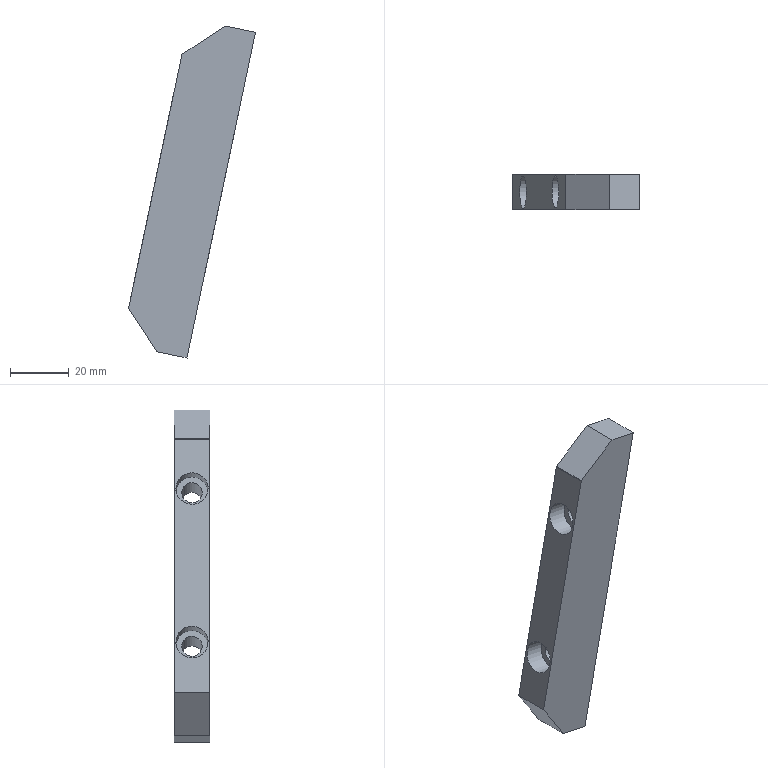Part | STEP file | BERCO_003 | 1 solid | 15 faces | box 43.278 x 12 x 113.233 mm | volume 26889 mm3 | plane 11 | cylinder 4 | commonest cylinder face diameters 7 x2 11 x2
STEP:
#1=CARTESIAN_POINT('',(0.,0.,0.));
#2=DIRECTION('',(0.,0.,1.));
#3=DIRECTION('',(1.,0.,0.));
#4=AXIS2_PLACEMENT_3D('',#1,#2,#3);
#5=CARTESIAN_POINT('',(1194.353,-560.013,65.597));
#6=VERTEX_POINT('',#5);
#7=CARTESIAN_POINT('',(1195.346,-562.65,70.321));
#8=DIRECTION('',(0.9786,0.,-0.2056));
#9=DIRECTION('',(0.2056,0.,0.9786));
#10=AXIS2_PLACEMENT_3D('',#7,#8,#9);
#11=CIRCLE('',#10,5.5);
#12=CARTESIAN_POINT('',(1196.066,-562.65,73.746));
#13=DIRECTION('',(0.9786,0.,-0.2056));
#14=DIRECTION('',(-0.2056,0.,-0.9786));
#15=AXIS2_PLACEMENT_3D('',#12,#13,#14);
#16=PLANE('',#15);
#17=CARTESIAN_POINT('',(3.5,0.));
#18=DIRECTION('',(-1.,0.));
#19=AXIS2_PLACEMENT_2D('',#17,#18);
#20=CIRCLE('',#19,5.5);
#21=(GEOMETRIC_REPRESENTATION_CONTEXT(2)PARAMETRIC_REPRESENTATION_CONTEXT()REPRESENTATION_CONTEXT('',''));
#22=DEFINITIONAL_REPRESENTATION('',(#20),#21);
#23=PCURVE('',#16,#22);
#24=CARTESIAN_POINT('',(1188.593,-562.65,71.74));
#25=DIRECTION('',(0.9786,0.,-0.2056));
#26=DIRECTION('',(0.1805,-0.4794,0.8588));
#27=AXIS2_PLACEMENT_3D('',#24,#25,#26);
#28=CYLINDRICAL_SURFACE('',#27,5.5);
#29=CARTESIAN_POINT('',(-0.5,6.9));
#30=DIRECTION('',(1.,0.));
#31=VECTOR('',#30,1.);
#32=LINE('',#29,#31);
#33=(GEOMETRIC_REPRESENTATION_CONTEXT(2)PARAMETRIC_REPRESENTATION_CONTEXT()REPRESENTATION_CONTEXT('',''));
#34=DEFINITIONAL_REPRESENTATION('',(#32),#33);
#35=PCURVE('',#28,#34);
#36=SURFACE_CURVE('',#11,(#23,#35),.PCURVE_S1.);
#37=EDGE_CURVE('',#6,#6,#36,.T.);
#38=ORIENTED_EDGE('',*,*,#37,.F.);
#39=EDGE_LOOP('',(#38));
#40=FACE_BOUND('',#39,.T.);
#41=CARTESIAN_POINT('',(1195.978,-564.328,73.327));
#42=VERTEX_POINT('',#41);
#43=CARTESIAN_POINT('',(1195.346,-562.65,70.321));
#44=DIRECTION('',(0.9786,0.,-0.2056));
#45=DIRECTION('',(0.2056,0.,0.9786));
#46=AXIS2_PLACEMENT_3D('',#43,#44,#45);
#47=CIRCLE('',#46,3.5);
#48=CARTESIAN_POINT('',(3.5,0.));
#49=DIRECTION('',(-1.,0.));
#50=AXIS2_PLACEMENT_2D('',#48,#49);
#51=CIRCLE('',#50,3.5);
#52=(GEOMETRIC_REPRESENTATION_CONTEXT(2)PARAMETRIC_REPRESENTATION_CONTEXT()REPRESENTATION_CONTEXT('',''));
#53=DEFINITIONAL_REPRESENTATION('',(#51),#52);
#54=PCURVE('',#16,#53);
#55=CARTESIAN_POINT('',(1188.593,-562.65,71.74));
#56=DIRECTION('',(0.9786,0.,-0.2056));
#57=DIRECTION('',(0.1805,-0.4794,0.8588));
#58=AXIS2_PLACEMENT_3D('',#55,#56,#57);
#59=CYLINDRICAL_SURFACE('',#58,3.5);
#60=CARTESIAN_POINT('',(-0.5,6.9));
#61=DIRECTION('',(1.,0.));
#62=VECTOR('',#61,1.);
#63=LINE('',#60,#62);
#64=(GEOMETRIC_REPRESENTATION_CONTEXT(2)PARAMETRIC_REPRESENTATION_CONTEXT()REPRESENTATION_CONTEXT('',''));
#65=DEFINITIONAL_REPRESENTATION('',(#63),#64);
#66=PCURVE('',#59,#65);
#67=SURFACE_CURVE('',#47,(#54,#66),.PCURVE_S1.);
#68=EDGE_CURVE('',#42,#42,#67,.T.);
#69=ORIENTED_EDGE('',*,*,#68,.T.);
#70=EDGE_LOOP('',(#69));
#71=FACE_BOUND('',#70,.T.);
#72=ADVANCED_FACE('',(#40,#71),#16,.F.);
#73=CARTESIAN_POINT('',(1211.636,-564.328,70.036));
#74=VERTEX_POINT('',#73);
#75=CARTESIAN_POINT('',(1211.004,-562.65,67.031));
#76=DIRECTION('',(0.9786,0.,-0.2056));
#77=DIRECTION('',(0.2056,0.,0.9786));
#78=AXIS2_PLACEMENT_3D('',#75,#76,#77);
#79=CIRCLE('',#78,3.5);
#80=CARTESIAN_POINT('',(-0.5,22.9));
#81=DIRECTION('',(1.,0.));
#82=VECTOR('',#81,1.);
#83=LINE('',#80,#82);
#84=(GEOMETRIC_REPRESENTATION_CONTEXT(2)PARAMETRIC_REPRESENTATION_CONTEXT()REPRESENTATION_CONTEXT('',''));
#85=DEFINITIONAL_REPRESENTATION('',(#83),#84);
#86=PCURVE('',#59,#85);
#87=CARTESIAN_POINT('',(1228.175,-556.65,148.746));
#88=DIRECTION('',(-0.9786,0.,0.2056));
#89=DIRECTION('',(0.2056,0.,0.9786));
#90=AXIS2_PLACEMENT_3D('',#87,#88,#89);
#91=PLANE('',#90);
#92=CARTESIAN_POINT('',(-80.,-6.));
#93=CARTESIAN_POINT('',(-80.,-12.062));
#94=CARTESIAN_POINT('',(-85.25,-9.031));
#95=CARTESIAN_POINT('',(-90.5,-6.));
#96=CARTESIAN_POINT('',(-85.25,-2.969));
#97=CARTESIAN_POINT('',(-80.,0.06218));
#98=CARTESIAN_POINT('',(-80.,-6.));
#99=(BOUNDED_CURVE()B_SPLINE_CURVE(2,(#92,#93,#94,#95,#96,#97,#98),.UNSPECIFIED.,.T.,.F.)B_SPLINE_CURVE_WITH_KNOTS((1,2,2,2,2,1),(-2.094,0.,2.094,4.189,6.283,8.378),.UNSPECIFIED.)CURVE()GEOMETRIC_REPRESENTATION_ITEM()RATIONAL_B_SPLINE_CURVE((1.,0.5,1.,0.5,1.,0.5,1.))REPRESENTATION_ITEM(''));
#100=(GEOMETRIC_REPRESENTATION_CONTEXT(2)PARAMETRIC_REPRESENTATION_CONTEXT()REPRESENTATION_CONTEXT('',''));
#101=DEFINITIONAL_REPRESENTATION('',(#99),#100);
#102=PCURVE('',#91,#101);
#103=SURFACE_CURVE('',#79,(#86,#102),.PCURVE_S1.);
#104=EDGE_CURVE('',#74,#74,#103,.T.);
#105=ORIENTED_EDGE('',*,*,#104,.F.);
#106=CARTESIAN_POINT('',(1195.978,-564.328,73.327));
#107=CARTESIAN_POINT('',(1211.636,-564.328,70.036));
#108=B_SPLINE_CURVE_WITH_KNOTS('',1,(#106,#107),.UNSPECIFIED.,.F.,.F.,(2,2),(6.9,22.9),.PIECEWISE_BEZIER_KNOTS.);
#109=CARTESIAN_POINT('',(0.,0.));
#110=DIRECTION('',(0.,1.));
#111=VECTOR('',#110,1.);
#112=LINE('',#109,#111);
#113=(GEOMETRIC_REPRESENTATION_CONTEXT(2)PARAMETRIC_REPRESENTATION_CONTEXT()REPRESENTATION_CONTEXT('',''));
#114=DEFINITIONAL_REPRESENTATION('',(#112),#113);
#115=PCURVE('',#59,#114);
#116=CARTESIAN_POINT('',(6.283,0.));
#117=DIRECTION('',(0.,1.));
#118=VECTOR('',#117,1.);
#119=LINE('',#116,#118);
#120=(GEOMETRIC_REPRESENTATION_CONTEXT(2)PARAMETRIC_REPRESENTATION_CONTEXT()REPRESENTATION_CONTEXT('',''));
#121=DEFINITIONAL_REPRESENTATION('',(#119),#120);
#122=PCURVE('',#59,#121);
#123=SEAM_CURVE('',#108,(#115,#122),.PCURVE_S1.);
#124=EDGE_CURVE('',#42,#74,#123,.T.);
#125=ORIENTED_EDGE('',*,*,#124,.F.);
#126=ORIENTED_EDGE('',*,*,#68,.T.);
#127=ORIENTED_EDGE('',*,*,#124,.T.);
#128=EDGE_LOOP('',(#105,#125,#126,#127));
#129=FACE_BOUND('',#128,.F.);
#130=ADVANCED_FACE('',(#129),#59,.F.);
#131=CARTESIAN_POINT('',(1187.503,-560.013,67.037));
#132=VERTEX_POINT('',#131);
#133=CARTESIAN_POINT('',(1188.496,-562.65,71.76));
#134=DIRECTION('',(0.9786,0.,-0.2056));
#135=DIRECTION('',(0.2056,0.,0.9786));
#136=AXIS2_PLACEMENT_3D('',#133,#134,#135);
#137=CIRCLE('',#136,5.5);
#138=CARTESIAN_POINT('',(-0.5,-0.1));
#139=DIRECTION('',(1.,0.));
#140=VECTOR('',#139,1.);
#141=LINE('',#138,#140);
#142=(GEOMETRIC_REPRESENTATION_CONTEXT(2)PARAMETRIC_REPRESENTATION_CONTEXT()REPRESENTATION_CONTEXT('',''));
#143=DEFINITIONAL_REPRESENTATION('',(#141),#142);
#144=PCURVE('',#28,#143);
#145=CARTESIAN_POINT('',(1184.383,-556.65,52.188));
#146=DIRECTION('',(-0.9786,0.,0.2056));
#147=DIRECTION('',(0.2056,0.,0.9786));
#148=AXIS2_PLACEMENT_3D('',#145,#146,#147);
#149=PLANE('',#148);
#150=CARTESIAN_POINT('',(25.5,-6.));
#151=CARTESIAN_POINT('',(25.5,-15.526));
#152=CARTESIAN_POINT('',(17.25,-10.763));
#153=CARTESIAN_POINT('',(9.,-6.));
#154=CARTESIAN_POINT('',(17.25,-1.237));
#155=CARTESIAN_POINT('',(25.5,3.526));
#156=CARTESIAN_POINT('',(25.5,-6.));
#157=(BOUNDED_CURVE()B_SPLINE_CURVE(2,(#150,#151,#152,#153,#154,#155,#156),.UNSPECIFIED.,.T.,.F.)B_SPLINE_CURVE_WITH_KNOTS((1,2,2,2,2,1),(-2.094,0.,2.094,4.189,6.283,8.378),.UNSPECIFIED.)CURVE()GEOMETRIC_REPRESENTATION_ITEM()RATIONAL_B_SPLINE_CURVE((1.,0.5,1.,0.5,1.,0.5,1.))REPRESENTATION_ITEM(''));
#158=(GEOMETRIC_REPRESENTATION_CONTEXT(2)PARAMETRIC_REPRESENTATION_CONTEXT()REPRESENTATION_CONTEXT('',''));
#159=DEFINITIONAL_REPRESENTATION('',(#157),#158);
#160=PCURVE('',#149,#159);
#161=SURFACE_CURVE('',#137,(#144,#160),.PCURVE_S1.);
#162=EDGE_CURVE('',#132,#132,#161,.T.);
#163=ORIENTED_EDGE('',*,*,#162,.T.);
#164=CARTESIAN_POINT('',(1187.503,-560.013,67.037));
#165=CARTESIAN_POINT('',(1194.353,-560.013,65.597));
#166=B_SPLINE_CURVE_WITH_KNOTS('',1,(#164,#165),.UNSPECIFIED.,.F.,.F.,(2,2),(-0.1,6.9),.PIECEWISE_BEZIER_KNOTS.);
#167=CARTESIAN_POINT('',(9.425,0.));
#168=DIRECTION('',(0.,1.));
#169=VECTOR('',#168,1.);
#170=LINE('',#167,#169);
#171=(GEOMETRIC_REPRESENTATION_CONTEXT(2)PARAMETRIC_REPRESENTATION_CONTEXT()REPRESENTATION_CONTEXT('',''));
#172=DEFINITIONAL_REPRESENTATION('',(#170),#171);
#173=PCURVE('',#28,#172);
#174=CARTESIAN_POINT('',(3.142,0.));
#175=DIRECTION('',(0.,1.));
#176=VECTOR('',#175,1.);
#177=LINE('',#174,#176);
#178=(GEOMETRIC_REPRESENTATION_CONTEXT(2)PARAMETRIC_REPRESENTATION_CONTEXT()REPRESENTATION_CONTEXT('',''));
#179=DEFINITIONAL_REPRESENTATION('',(#177),#178);
#180=PCURVE('',#28,#179);
#181=SEAM_CURVE('',#166,(#173,#180),.PCURVE_S1.);
#182=EDGE_CURVE('',#132,#6,#181,.T.);
#183=ORIENTED_EDGE('',*,*,#182,.T.);
#184=ORIENTED_EDGE('',*,*,#37,.F.);
#185=ORIENTED_EDGE('',*,*,#182,.F.);
#186=EDGE_LOOP('',(#163,#183,#184,#185));
#187=FACE_BOUND('',#186,.F.);
#188=ADVANCED_FACE('',(#187),#28,.F.);
#189=CARTESIAN_POINT('',(1228.175,-568.65,148.746));
#190=VERTEX_POINT('',#189);
#191=CARTESIAN_POINT('',(1204.835,-568.65,37.672));
#192=VERTEX_POINT('',#191);
#193=CARTESIAN_POINT('',(1228.175,-568.65,148.746));
#194=DIRECTION('',(-0.2056,0.,-0.9786));
#195=VECTOR('',#194,1.);
#196=LINE('',#193,#195);
#197=CARTESIAN_POINT('',(0.,-12.));
#198=DIRECTION('',(-1.,0.));
#199=VECTOR('',#198,1.);
#200=LINE('',#197,#199);
#201=(GEOMETRIC_REPRESENTATION_CONTEXT(2)PARAMETRIC_REPRESENTATION_CONTEXT()REPRESENTATION_CONTEXT('',''));
#202=DEFINITIONAL_REPRESENTATION('',(#200),#201);
#203=PCURVE('',#91,#202);
#204=CARTESIAN_POINT('',(0.,-568.65,0.));
#205=DIRECTION('',(0.,1.,0.));
#206=DIRECTION('',(0.,0.,1.));
#207=AXIS2_PLACEMENT_3D('',#204,#205,#206);
#208=PLANE('',#207);
#209=CARTESIAN_POINT('',(148.746,1228.175));
#210=DIRECTION('',(-0.9786,-0.2056));
#211=VECTOR('',#210,1.);
#212=LINE('',#209,#211);
#213=(GEOMETRIC_REPRESENTATION_CONTEXT(2)PARAMETRIC_REPRESENTATION_CONTEXT()REPRESENTATION_CONTEXT('',''));
#214=DEFINITIONAL_REPRESENTATION('',(#212),#213);
#215=PCURVE('',#208,#214);
#216=SURFACE_CURVE('',#196,(#203,#215),.PCURVE_S1.);
#217=EDGE_CURVE('',#190,#192,#216,.T.);
#218=ORIENTED_EDGE('',*,*,#217,.T.);
#219=CARTESIAN_POINT('',(1204.835,-556.65,37.672));
#220=VERTEX_POINT('',#219);
#221=CARTESIAN_POINT('',(1204.835,-556.65,37.672));
#222=DIRECTION('',(0.,-1.,0.));
#223=VECTOR('',#222,1.);
#224=LINE('',#221,#223);
#225=CARTESIAN_POINT('',(-113.5,0.));
#226=DIRECTION('',(0.,-1.));
#227=VECTOR('',#226,1.);
#228=LINE('',#225,#227);
#229=(GEOMETRIC_REPRESENTATION_CONTEXT(2)PARAMETRIC_REPRESENTATION_CONTEXT()REPRESENTATION_CONTEXT('',''));
#230=DEFINITIONAL_REPRESENTATION('',(#228),#229);
#231=PCURVE('',#91,#230);
#232=CARTESIAN_POINT('',(1192.113,-556.65,40.345));
#233=DIRECTION('',(-0.2056,0.,-0.9786));
#234=DIRECTION('',(-0.9786,0.,0.2056));
#235=AXIS2_PLACEMENT_3D('',#232,#233,#234);
#236=PLANE('',#235);
#237=CARTESIAN_POINT('',(-13.,0.));
#238=DIRECTION('',(0.,-1.));
#239=VECTOR('',#238,1.);
#240=LINE('',#237,#239);
#241=(GEOMETRIC_REPRESENTATION_CONTEXT(2)PARAMETRIC_REPRESENTATION_CONTEXT()REPRESENTATION_CONTEXT('',''));
#242=DEFINITIONAL_REPRESENTATION('',(#240),#241);
#243=PCURVE('',#236,#242);
#244=SURFACE_CURVE('',#224,(#231,#243),.PCURVE_S1.);
#245=EDGE_CURVE('',#220,#192,#244,.T.);
#246=ORIENTED_EDGE('',*,*,#245,.F.);
#247=CARTESIAN_POINT('',(1228.175,-556.65,148.746));
#248=VERTEX_POINT('',#247);
#249=CARTESIAN_POINT('',(1228.175,-556.65,148.746));
#250=DIRECTION('',(-0.2056,0.,-0.9786));
#251=VECTOR('',#250,1.);
#252=LINE('',#249,#251);
#253=CARTESIAN_POINT('',(0.,0.));
#254=DIRECTION('',(-1.,0.));
#255=VECTOR('',#254,1.);
#256=LINE('',#253,#255);
#257=(GEOMETRIC_REPRESENTATION_CONTEXT(2)PARAMETRIC_REPRESENTATION_CONTEXT()REPRESENTATION_CONTEXT('',''));
#258=DEFINITIONAL_REPRESENTATION('',(#256),#257);
#259=PCURVE('',#91,#258);
#260=CARTESIAN_POINT('',(0.,-556.65,0.));
#261=DIRECTION('',(0.,1.,0.));
#262=DIRECTION('',(0.,0.,1.));
#263=AXIS2_PLACEMENT_3D('',#260,#261,#262);
#264=PLANE('',#263);
#265=CARTESIAN_POINT('',(148.746,1228.175));
#266=DIRECTION('',(-0.9786,-0.2056));
#267=VECTOR('',#266,1.);
#268=LINE('',#265,#267);
#269=(GEOMETRIC_REPRESENTATION_CONTEXT(2)PARAMETRIC_REPRESENTATION_CONTEXT()REPRESENTATION_CONTEXT('',''));
#270=DEFINITIONAL_REPRESENTATION('',(#268),#269);
#271=PCURVE('',#264,#270);
#272=SURFACE_CURVE('',#252,(#259,#271),.PCURVE_S1.);
#273=EDGE_CURVE('',#248,#220,#272,.T.);
#274=ORIENTED_EDGE('',*,*,#273,.F.);
#275=CARTESIAN_POINT('',(1228.175,-556.65,148.746));
#276=DIRECTION('',(0.,-1.,0.));
#277=VECTOR('',#276,1.);
#278=LINE('',#275,#277);
#279=CARTESIAN_POINT('',(0.,0.));
#280=DIRECTION('',(0.,-1.));
#281=VECTOR('',#280,1.);
#282=LINE('',#279,#281);
#283=(GEOMETRIC_REPRESENTATION_CONTEXT(2)PARAMETRIC_REPRESENTATION_CONTEXT()REPRESENTATION_CONTEXT('',''));
#284=DEFINITIONAL_REPRESENTATION('',(#282),#283);
#285=PCURVE('',#91,#284);
#286=CARTESIAN_POINT('',(1205.667,-556.65,153.476));
#287=DIRECTION('',(-0.2056,0.,-0.9786));
#288=DIRECTION('',(-0.9786,0.,0.2056));
#289=AXIS2_PLACEMENT_3D('',#286,#287,#288);
#290=PLANE('',#289);
#291=CARTESIAN_POINT('',(-23.,0.));
#292=DIRECTION('',(0.,-1.));
#293=VECTOR('',#292,1.);
#294=LINE('',#291,#293);
#295=(GEOMETRIC_REPRESENTATION_CONTEXT(2)PARAMETRIC_REPRESENTATION_CONTEXT()REPRESENTATION_CONTEXT('',''));
#296=DEFINITIONAL_REPRESENTATION('',(#294),#295);
#297=PCURVE('',#290,#296);
#298=SURFACE_CURVE('',#278,(#285,#297),.PCURVE_S1.);
#299=EDGE_CURVE('',#248,#190,#298,.T.);
#300=ORIENTED_EDGE('',*,*,#299,.T.);
#301=EDGE_LOOP('',(#218,#246,#274,#300));
#302=FACE_BOUND('',#301,.T.);
#303=CARTESIAN_POINT('',(1222.638,-564.328,122.393));
#304=VERTEX_POINT('',#303);
#305=CARTESIAN_POINT('',(1222.006,-562.65,119.387));
#306=DIRECTION('',(-0.9786,0.,0.2056));
#307=DIRECTION('',(0.2056,0.,0.9786));
#308=AXIS2_PLACEMENT_3D('',#305,#306,#307);
#309=CIRCLE('',#308,3.5);
#310=CARTESIAN_POINT('',(-30.,-6.));
#311=DIRECTION('',(1.,0.));
#312=AXIS2_PLACEMENT_2D('',#310,#311);
#313=CIRCLE('',#312,3.5);
#314=(GEOMETRIC_REPRESENTATION_CONTEXT(2)PARAMETRIC_REPRESENTATION_CONTEXT()REPRESENTATION_CONTEXT('',''));
#315=DEFINITIONAL_REPRESENTATION('',(#313),#314);
#316=PCURVE('',#91,#315);
#317=CARTESIAN_POINT('',(1199.595,-562.65,124.096));
#318=DIRECTION('',(0.9786,0.,-0.2056));
#319=DIRECTION('',(0.1805,-0.4794,0.8588));
#320=AXIS2_PLACEMENT_3D('',#317,#318,#319);
#321=CYLINDRICAL_SURFACE('',#320,3.5);
#322=CARTESIAN_POINT('',(12.066,22.9));
#323=DIRECTION('',(-1.,0.));
#324=VECTOR('',#323,1.);
#325=LINE('',#322,#324);
#326=(GEOMETRIC_REPRESENTATION_CONTEXT(2)PARAMETRIC_REPRESENTATION_CONTEXT()REPRESENTATION_CONTEXT('',''));
#327=DEFINITIONAL_REPRESENTATION('',(#325),#326);
#328=PCURVE('',#321,#327);
#329=SURFACE_CURVE('',#309,(#316,#328),.PCURVE_S1.);
#330=EDGE_CURVE('',#304,#304,#329,.T.);
#331=ORIENTED_EDGE('',*,*,#330,.T.);
#332=EDGE_LOOP('',(#331));
#333=FACE_BOUND('',#332,.T.);
#334=ORIENTED_EDGE('',*,*,#104,.F.);
#335=EDGE_LOOP('',(#334));
#336=FACE_BOUND('',#335,.T.);
#337=ADVANCED_FACE('',(#302,#333,#336),#91,.F.);
#338=CARTESIAN_POINT('',(1207.34,-565.287,127.401));
#339=VERTEX_POINT('',#338);
#340=CARTESIAN_POINT('',(1206.348,-562.65,122.677));
#341=DIRECTION('',(0.9786,0.,-0.2056));
#342=DIRECTION('',(0.2056,0.,0.9786));
#343=AXIS2_PLACEMENT_3D('',#340,#341,#342);
#344=CIRCLE('',#343,5.5);
#345=CARTESIAN_POINT('',(1196.066,-562.65,73.746));
#346=DIRECTION('',(0.9786,0.,-0.2056));
#347=DIRECTION('',(-0.2056,0.,-0.9786));
#348=AXIS2_PLACEMENT_3D('',#345,#346,#347);
#349=PLANE('',#348);
#350=CARTESIAN_POINT('',(-50.,0.));
#351=DIRECTION('',(-1.,0.));
#352=AXIS2_PLACEMENT_2D('',#350,#351);
#353=CIRCLE('',#352,5.5);
#354=(GEOMETRIC_REPRESENTATION_CONTEXT(2)PARAMETRIC_REPRESENTATION_CONTEXT()REPRESENTATION_CONTEXT('',''));
#355=DEFINITIONAL_REPRESENTATION('',(#353),#354);
#356=PCURVE('',#349,#355);
#357=CARTESIAN_POINT('',(1199.595,-562.65,124.096));
#358=DIRECTION('',(0.9786,0.,-0.2056));
#359=DIRECTION('',(0.1805,-0.4794,0.8588));
#360=AXIS2_PLACEMENT_3D('',#357,#358,#359);
#361=CYLINDRICAL_SURFACE('',#360,5.5);
#362=CARTESIAN_POINT('',(-0.5,6.9));
#363=DIRECTION('',(1.,0.));
#364=VECTOR('',#363,1.);
#365=LINE('',#362,#364);
#366=(GEOMETRIC_REPRESENTATION_CONTEXT(2)PARAMETRIC_REPRESENTATION_CONTEXT()REPRESENTATION_CONTEXT('',''));
#367=DEFINITIONAL_REPRESENTATION('',(#365),#366);
#368=PCURVE('',#361,#367);
#369=SURFACE_CURVE('',#344,(#356,#368),.PCURVE_S1.);
#370=EDGE_CURVE('',#339,#339,#369,.T.);
#371=ORIENTED_EDGE('',*,*,#370,.F.);
#372=EDGE_LOOP('',(#371));
#373=FACE_BOUND('',#372,.T.);
#374=CARTESIAN_POINT('',(1206.98,-564.328,125.683));
#375=VERTEX_POINT('',#374);
#376=CARTESIAN_POINT('',(1206.348,-562.65,122.677));
#377=DIRECTION('',(0.9786,0.,-0.2056));
#378=DIRECTION('',(0.2056,0.,0.9786));
#379=AXIS2_PLACEMENT_3D('',#376,#377,#378);
#380=CIRCLE('',#379,3.5);
#381=CARTESIAN_POINT('',(-50.,0.));
#382=DIRECTION('',(-1.,0.));
#383=AXIS2_PLACEMENT_2D('',#381,#382);
#384=CIRCLE('',#383,3.5);
#385=(GEOMETRIC_REPRESENTATION_CONTEXT(2)PARAMETRIC_REPRESENTATION_CONTEXT()REPRESENTATION_CONTEXT('',''));
#386=DEFINITIONAL_REPRESENTATION('',(#384),#385);
#387=PCURVE('',#349,#386);
#388=CARTESIAN_POINT('',(-0.5,6.9));
#389=DIRECTION('',(1.,0.));
#390=VECTOR('',#389,1.);
#391=LINE('',#388,#390);
#392=(GEOMETRIC_REPRESENTATION_CONTEXT(2)PARAMETRIC_REPRESENTATION_CONTEXT()REPRESENTATION_CONTEXT('',''));
#393=DEFINITIONAL_REPRESENTATION('',(#391),#392);
#394=PCURVE('',#321,#393);
#395=SURFACE_CURVE('',#380,(#387,#394),.PCURVE_S1.);
#396=EDGE_CURVE('',#375,#375,#395,.T.);
#397=ORIENTED_EDGE('',*,*,#396,.T.);
#398=EDGE_LOOP('',(#397));
#399=FACE_BOUND('',#398,.T.);
#400=ADVANCED_FACE('',(#373,#399),#349,.F.);
#401=CARTESIAN_POINT('',(1200.49,-565.287,128.84));
#402=VERTEX_POINT('',#401);
#403=CARTESIAN_POINT('',(1199.497,-562.65,124.117));
#404=DIRECTION('',(0.9786,0.,-0.2056));
#405=DIRECTION('',(0.2056,0.,0.9786));
#406=AXIS2_PLACEMENT_3D('',#403,#404,#405);
#407=CIRCLE('',#406,5.5);
#408=CARTESIAN_POINT('',(-0.5,-0.1));
#409=DIRECTION('',(1.,0.));
#410=VECTOR('',#409,1.);
#411=LINE('',#408,#410);
#412=(GEOMETRIC_REPRESENTATION_CONTEXT(2)PARAMETRIC_REPRESENTATION_CONTEXT()REPRESENTATION_CONTEXT('',''));
#413=DEFINITIONAL_REPRESENTATION('',(#411),#412);
#414=PCURVE('',#361,#413);
#415=CARTESIAN_POINT('',(79.,-6.));
#416=CARTESIAN_POINT('',(79.,-15.526));
#417=CARTESIAN_POINT('',(70.75,-10.763));
#418=CARTESIAN_POINT('',(62.5,-6.));
#419=CARTESIAN_POINT('',(70.75,-1.237));
#420=CARTESIAN_POINT('',(79.,3.526));
#421=CARTESIAN_POINT('',(79.,-6.));
#422=(BOUNDED_CURVE()B_SPLINE_CURVE(2,(#415,#416,#417,#418,#419,#420,#421),.UNSPECIFIED.,.T.,.F.)B_SPLINE_CURVE_WITH_KNOTS((1,2,2,2,2,1),(-2.094,0.,2.094,4.189,6.283,8.378),.UNSPECIFIED.)CURVE()GEOMETRIC_REPRESENTATION_ITEM()RATIONAL_B_SPLINE_CURVE((1.,0.5,1.,0.5,1.,0.5,1.))REPRESENTATION_ITEM(''));
#423=(GEOMETRIC_REPRESENTATION_CONTEXT(2)PARAMETRIC_REPRESENTATION_CONTEXT()REPRESENTATION_CONTEXT('',''));
#424=DEFINITIONAL_REPRESENTATION('',(#422),#423);
#425=PCURVE('',#149,#424);
#426=SURFACE_CURVE('',#407,(#414,#425),.PCURVE_S1.);
#427=EDGE_CURVE('',#402,#402,#426,.T.);
#428=ORIENTED_EDGE('',*,*,#427,.T.);
#429=CARTESIAN_POINT('',(1200.49,-565.287,128.84));
#430=CARTESIAN_POINT('',(1207.34,-565.287,127.401));
#431=B_SPLINE_CURVE_WITH_KNOTS('',1,(#429,#430),.UNSPECIFIED.,.F.,.F.,(2,2),(-0.1,6.9),.PIECEWISE_BEZIER_KNOTS.);
#432=CARTESIAN_POINT('',(6.283,0.));
#433=DIRECTION('',(0.,1.));
#434=VECTOR('',#433,1.);
#435=LINE('',#432,#434);
#436=(GEOMETRIC_REPRESENTATION_CONTEXT(2)PARAMETRIC_REPRESENTATION_CONTEXT()REPRESENTATION_CONTEXT('',''));
#437=DEFINITIONAL_REPRESENTATION('',(#435),#436);
#438=PCURVE('',#361,#437);
#439=CARTESIAN_POINT('',(0.,0.));
#440=DIRECTION('',(0.,1.));
#441=VECTOR('',#440,1.);
#442=LINE('',#439,#441);
#443=(GEOMETRIC_REPRESENTATION_CONTEXT(2)PARAMETRIC_REPRESENTATION_CONTEXT()REPRESENTATION_CONTEXT('',''));
#444=DEFINITIONAL_REPRESENTATION('',(#442),#443);
#445=PCURVE('',#361,#444);
#446=SEAM_CURVE('',#431,(#438,#445),.PCURVE_S1.);
#447=EDGE_CURVE('',#402,#339,#446,.T.);
#448=ORIENTED_EDGE('',*,*,#447,.T.);
#449=ORIENTED_EDGE('',*,*,#370,.F.);
#450=ORIENTED_EDGE('',*,*,#447,.F.);
#451=EDGE_LOOP('',(#428,#448,#449,#450));
#452=FACE_BOUND('',#451,.F.);
#453=ADVANCED_FACE('',(#452),#361,.F.);
#454=ORIENTED_EDGE('',*,*,#330,.T.);
#455=CARTESIAN_POINT('',(1206.98,-564.328,125.683));
#456=CARTESIAN_POINT('',(1222.638,-564.328,122.393));
#457=B_SPLINE_CURVE_WITH_KNOTS('',1,(#455,#456),.UNSPECIFIED.,.F.,.F.,(2,2),(6.9,22.9),.PIECEWISE_BEZIER_KNOTS.);
#458=CARTESIAN_POINT('',(0.,0.));
#459=DIRECTION('',(0.,1.));
#460=VECTOR('',#459,1.);
#461=LINE('',#458,#460);
#462=(GEOMETRIC_REPRESENTATION_CONTEXT(2)PARAMETRIC_REPRESENTATION_CONTEXT()REPRESENTATION_CONTEXT('',''));
#463=DEFINITIONAL_REPRESENTATION('',(#461),#462);
#464=PCURVE('',#321,#463);
#465=CARTESIAN_POINT('',(6.283,0.));
#466=DIRECTION('',(0.,1.));
#467=VECTOR('',#466,1.);
#468=LINE('',#465,#467);
#469=(GEOMETRIC_REPRESENTATION_CONTEXT(2)PARAMETRIC_REPRESENTATION_CONTEXT()REPRESENTATION_CONTEXT('',''));
#470=DEFINITIONAL_REPRESENTATION('',(#468),#469);
#471=PCURVE('',#321,#470);
#472=SEAM_CURVE('',#457,(#464,#471),.PCURVE_S1.);
#473=EDGE_CURVE('',#375,#304,#472,.T.);
#474=ORIENTED_EDGE('',*,*,#473,.F.);
#475=ORIENTED_EDGE('',*,*,#396,.T.);
#476=ORIENTED_EDGE('',*,*,#473,.T.);
#477=EDGE_LOOP('',(#454,#474,#475,#476));
#478=FACE_BOUND('',#477,.F.);
#479=ADVANCED_FACE('',(#478),#321,.F.);
#480=CARTESIAN_POINT('',(1217.9,-556.65,150.905));
#481=VERTEX_POINT('',#480);
#482=CARTESIAN_POINT('',(1217.9,-568.65,150.905));
#483=VERTEX_POINT('',#482);
#484=CARTESIAN_POINT('',(1217.9,-556.65,150.905));
#485=DIRECTION('',(0.,-1.,0.));
#486=VECTOR('',#485,1.);
#487=LINE('',#484,#486);
#488=CARTESIAN_POINT('',(-12.5,0.));
#489=DIRECTION('',(0.,-1.));
#490=VECTOR('',#489,1.);
#491=LINE('',#488,#490);
#492=(GEOMETRIC_REPRESENTATION_CONTEXT(2)PARAMETRIC_REPRESENTATION_CONTEXT()REPRESENTATION_CONTEXT('',''));
#493=DEFINITIONAL_REPRESENTATION('',(#491),#492);
#494=PCURVE('',#290,#493);
#495=CARTESIAN_POINT('',(1203.096,-554.25,141.243));
#496=DIRECTION('',(-0.5466,0.,0.8374));
#497=DIRECTION('',(0.8374,0.,0.5466));
#498=AXIS2_PLACEMENT_3D('',#495,#496,#497);
#499=PLANE('',#498);
#500=CARTESIAN_POINT('',(17.678,-2.4));
#501=DIRECTION('',(0.,-1.));
#502=VECTOR('',#501,1.);
#503=LINE('',#500,#502);
#504=(GEOMETRIC_REPRESENTATION_CONTEXT(2)PARAMETRIC_REPRESENTATION_CONTEXT()REPRESENTATION_CONTEXT('',''));
#505=DEFINITIONAL_REPRESENTATION('',(#503),#504);
#506=PCURVE('',#499,#505);
#507=SURFACE_CURVE('',#487,(#494,#506),.PCURVE_S1.);
#508=EDGE_CURVE('',#481,#483,#507,.T.);
#509=ORIENTED_EDGE('',*,*,#508,.T.);
#510=CARTESIAN_POINT('',(1217.9,-568.65,150.905));
#511=DIRECTION('',(0.9786,0.,-0.2056));
#512=VECTOR('',#511,1.);
#513=LINE('',#510,#512);
#514=CARTESIAN_POINT('',(-12.5,-12.));
#515=DIRECTION('',(-1.,0.));
#516=VECTOR('',#515,1.);
#517=LINE('',#514,#516);
#518=(GEOMETRIC_REPRESENTATION_CONTEXT(2)PARAMETRIC_REPRESENTATION_CONTEXT()REPRESENTATION_CONTEXT('',''));
#519=DEFINITIONAL_REPRESENTATION('',(#517),#518);
#520=PCURVE('',#290,#519);
#521=CARTESIAN_POINT('',(150.905,1217.9));
#522=DIRECTION('',(-0.2056,0.9786));
#523=VECTOR('',#522,1.);
#524=LINE('',#521,#523);
#525=(GEOMETRIC_REPRESENTATION_CONTEXT(2)PARAMETRIC_REPRESENTATION_CONTEXT()REPRESENTATION_CONTEXT('',''));
#526=DEFINITIONAL_REPRESENTATION('',(#524),#525);
#527=PCURVE('',#208,#526);
#528=SURFACE_CURVE('',#513,(#520,#527),.PCURVE_S1.);
#529=EDGE_CURVE('',#483,#190,#528,.T.);
#530=ORIENTED_EDGE('',*,*,#529,.T.);
#531=ORIENTED_EDGE('',*,*,#299,.F.);
#532=CARTESIAN_POINT('',(1217.9,-556.65,150.905));
#533=DIRECTION('',(0.9786,0.,-0.2056));
#534=VECTOR('',#533,1.);
#535=LINE('',#532,#534);
#536=CARTESIAN_POINT('',(-12.5,0.));
#537=DIRECTION('',(-1.,0.));
#538=VECTOR('',#537,1.);
#539=LINE('',#536,#538);
#540=(GEOMETRIC_REPRESENTATION_CONTEXT(2)PARAMETRIC_REPRESENTATION_CONTEXT()REPRESENTATION_CONTEXT('',''));
#541=DEFINITIONAL_REPRESENTATION('',(#539),#540);
#542=PCURVE('',#290,#541);
#543=CARTESIAN_POINT('',(150.905,1217.9));
#544=DIRECTION('',(-0.2056,0.9786));
#545=VECTOR('',#544,1.);
#546=LINE('',#543,#545);
#547=(GEOMETRIC_REPRESENTATION_CONTEXT(2)PARAMETRIC_REPRESENTATION_CONTEXT()REPRESENTATION_CONTEXT('',''));
#548=DEFINITIONAL_REPRESENTATION('',(#546),#547);
#549=PCURVE('',#264,#548);
#550=SURFACE_CURVE('',#535,(#542,#549),.PCURVE_S1.);
#551=EDGE_CURVE('',#481,#248,#550,.T.);
#552=ORIENTED_EDGE('',*,*,#551,.F.);
#553=EDGE_LOOP('',(#509,#530,#531,#552));
#554=FACE_BOUND('',#553,.T.);
#555=ADVANCED_FACE('',(#554),#290,.F.);
#556=CARTESIAN_POINT('',(1203.041,-556.65,140.978));
#557=VERTEX_POINT('',#556);
#558=CARTESIAN_POINT('',(1203.096,-556.65,141.243));
#559=VERTEX_POINT('',#558);
#560=CARTESIAN_POINT('',(1203.041,-556.65,140.978));
#561=DIRECTION('',(0.2056,0.,0.9786));
#562=VECTOR('',#561,1.);
#563=LINE('',#560,#562);
#564=CARTESIAN_POINT('',(1184.383,-556.65,52.188));
#565=DIRECTION('',(-0.9786,0.,0.2056));
#566=DIRECTION('',(0.2056,0.,0.9786));
#567=AXIS2_PLACEMENT_3D('',#564,#565,#566);
#568=PLANE('',#567);
#569=CARTESIAN_POINT('',(90.729,0.));
#570=DIRECTION('',(1.,0.));
#571=VECTOR('',#570,1.);
#572=LINE('',#569,#571);
#573=(GEOMETRIC_REPRESENTATION_CONTEXT(2)PARAMETRIC_REPRESENTATION_CONTEXT()REPRESENTATION_CONTEXT('',''));
#574=DEFINITIONAL_REPRESENTATION('',(#572),#573);
#575=PCURVE('',#568,#574);
#576=CARTESIAN_POINT('',(140.978,1203.041));
#577=DIRECTION('',(0.9786,0.2056));
#578=VECTOR('',#577,1.);
#579=LINE('',#576,#578);
#580=(GEOMETRIC_REPRESENTATION_CONTEXT(2)PARAMETRIC_REPRESENTATION_CONTEXT()REPRESENTATION_CONTEXT('',''));
#581=DEFINITIONAL_REPRESENTATION('',(#579),#580);
#582=PCURVE('',#264,#581);
#583=SURFACE_CURVE('',#563,(#575,#582),.PCURVE_S1.);
#584=EDGE_CURVE('',#557,#559,#583,.T.);
#585=ORIENTED_EDGE('',*,*,#584,.F.);
#586=CARTESIAN_POINT('',(1203.041,-568.65,140.978));
#587=VERTEX_POINT('',#586);
#588=CARTESIAN_POINT('',(1203.041,-556.65,140.978));
#589=DIRECTION('',(0.,-1.,0.));
#590=VECTOR('',#589,1.);
#591=LINE('',#588,#590);
#592=CARTESIAN_POINT('',(90.729,0.));
#593=DIRECTION('',(0.,-1.));
#594=VECTOR('',#593,1.);
#595=LINE('',#592,#594);
#596=(GEOMETRIC_REPRESENTATION_CONTEXT(2)PARAMETRIC_REPRESENTATION_CONTEXT()REPRESENTATION_CONTEXT('',''));
#597=DEFINITIONAL_REPRESENTATION('',(#595),#596);
#598=PCURVE('',#568,#597);
#599=CARTESIAN_POINT('',(90.729,0.));
#600=DIRECTION('',(0.,-1.));
#601=VECTOR('',#600,1.);
#602=LINE('',#599,#601);
#603=(GEOMETRIC_REPRESENTATION_CONTEXT(2)PARAMETRIC_REPRESENTATION_CONTEXT()REPRESENTATION_CONTEXT('',''));
#604=DEFINITIONAL_REPRESENTATION('',(#602),#603);
#605=PCURVE('',#149,#604);
#606=SURFACE_CURVE('',#591,(#598,#605),.PCURVE_S1.);
#607=EDGE_CURVE('',#557,#587,#606,.T.);
#608=ORIENTED_EDGE('',*,*,#607,.T.);
#609=CARTESIAN_POINT('',(1203.096,-568.65,141.243));
#610=VERTEX_POINT('',#609);
#611=CARTESIAN_POINT('',(1203.041,-568.65,140.978));
#612=DIRECTION('',(0.2056,0.,0.9786));
#613=VECTOR('',#612,1.);
#614=LINE('',#611,#613);
#615=CARTESIAN_POINT('',(90.729,-12.));
#616=DIRECTION('',(1.,0.));
#617=VECTOR('',#616,1.);
#618=LINE('',#615,#617);
#619=(GEOMETRIC_REPRESENTATION_CONTEXT(2)PARAMETRIC_REPRESENTATION_CONTEXT()REPRESENTATION_CONTEXT('',''));
#620=DEFINITIONAL_REPRESENTATION('',(#618),#619);
#621=PCURVE('',#568,#620);
#622=CARTESIAN_POINT('',(140.978,1203.041));
#623=DIRECTION('',(0.9786,0.2056));
#624=VECTOR('',#623,1.);
#625=LINE('',#622,#624);
#626=(GEOMETRIC_REPRESENTATION_CONTEXT(2)PARAMETRIC_REPRESENTATION_CONTEXT()REPRESENTATION_CONTEXT('',''));
#627=DEFINITIONAL_REPRESENTATION('',(#625),#626);
#628=PCURVE('',#208,#627);
#629=SURFACE_CURVE('',#614,(#621,#628),.PCURVE_S1.);
#630=EDGE_CURVE('',#587,#610,#629,.T.);
#631=ORIENTED_EDGE('',*,*,#630,.T.);
#632=CARTESIAN_POINT('',(1203.096,-556.65,141.243));
#633=DIRECTION('',(0.,-1.,0.));
#634=VECTOR('',#633,1.);
#635=LINE('',#632,#634);
#636=CARTESIAN_POINT('',(91.,0.));
#637=DIRECTION('',(0.,-1.));
#638=VECTOR('',#637,1.);
#639=LINE('',#636,#638);
#640=(GEOMETRIC_REPRESENTATION_CONTEXT(2)PARAMETRIC_REPRESENTATION_CONTEXT()REPRESENTATION_CONTEXT('',''));
#641=DEFINITIONAL_REPRESENTATION('',(#639),#640);
#642=PCURVE('',#568,#641);
#643=CARTESIAN_POINT('',(0.,-2.4));
#644=DIRECTION('',(0.,-1.));
#645=VECTOR('',#644,1.);
#646=LINE('',#643,#645);
#647=(GEOMETRIC_REPRESENTATION_CONTEXT(2)PARAMETRIC_REPRESENTATION_CONTEXT()REPRESENTATION_CONTEXT('',''));
#648=DEFINITIONAL_REPRESENTATION('',(#646),#647);
#649=PCURVE('',#499,#648);
#650=SURFACE_CURVE('',#635,(#642,#649),.PCURVE_S1.);
#651=EDGE_CURVE('',#559,#610,#650,.T.);
#652=ORIENTED_EDGE('',*,*,#651,.F.);
#653=EDGE_LOOP('',(#585,#608,#631,#652));
#654=FACE_BOUND('',#653,.T.);
#655=ADVANCED_FACE('',(#654),#568,.T.);
#656=CARTESIAN_POINT('',(1203.096,-568.65,141.243));
#657=DIRECTION('',(0.8374,0.,0.5466));
#658=VECTOR('',#657,1.);
#659=LINE('',#656,#658);
#660=CARTESIAN_POINT('',(-0.000000001,-14.4));
#661=DIRECTION('',(1.,0.));
#662=VECTOR('',#661,1.);
#663=LINE('',#660,#662);
#664=(GEOMETRIC_REPRESENTATION_CONTEXT(2)PARAMETRIC_REPRESENTATION_CONTEXT()REPRESENTATION_CONTEXT('',''));
#665=DEFINITIONAL_REPRESENTATION('',(#663),#664);
#666=PCURVE('',#499,#665);
#667=CARTESIAN_POINT('',(141.243,1203.096));
#668=DIRECTION('',(0.5466,0.8374));
#669=VECTOR('',#668,1.);
#670=LINE('',#667,#669);
#671=(GEOMETRIC_REPRESENTATION_CONTEXT(2)PARAMETRIC_REPRESENTATION_CONTEXT()REPRESENTATION_CONTEXT('',''));
#672=DEFINITIONAL_REPRESENTATION('',(#670),#671);
#673=PCURVE('',#208,#672);
#674=SURFACE_CURVE('',#659,(#666,#673),.PCURVE_S1.);
#675=EDGE_CURVE('',#610,#483,#674,.T.);
#676=ORIENTED_EDGE('',*,*,#675,.T.);
#677=ORIENTED_EDGE('',*,*,#508,.F.);
#678=CARTESIAN_POINT('',(1203.096,-556.65,141.243));
#679=DIRECTION('',(0.8374,0.,0.5466));
#680=VECTOR('',#679,1.);
#681=LINE('',#678,#680);
#682=CARTESIAN_POINT('',(-0.000000001,-2.4));
#683=DIRECTION('',(1.,0.));
#684=VECTOR('',#683,1.);
#685=LINE('',#682,#684);
#686=(GEOMETRIC_REPRESENTATION_CONTEXT(2)PARAMETRIC_REPRESENTATION_CONTEXT()REPRESENTATION_CONTEXT('',''));
#687=DEFINITIONAL_REPRESENTATION('',(#685),#686);
#688=PCURVE('',#499,#687);
#689=CARTESIAN_POINT('',(141.243,1203.096));
#690=DIRECTION('',(0.5466,0.8374));
#691=VECTOR('',#690,1.);
#692=LINE('',#689,#691);
#693=(GEOMETRIC_REPRESENTATION_CONTEXT(2)PARAMETRIC_REPRESENTATION_CONTEXT()REPRESENTATION_CONTEXT('',''));
#694=DEFINITIONAL_REPRESENTATION('',(#692),#693);
#695=PCURVE('',#264,#694);
#696=SURFACE_CURVE('',#681,(#688,#695),.PCURVE_S1.);
#697=EDGE_CURVE('',#559,#481,#696,.T.);
#698=ORIENTED_EDGE('',*,*,#697,.F.);
#699=ORIENTED_EDGE('',*,*,#651,.T.);
#700=EDGE_LOOP('',(#676,#677,#698,#699));
#701=FACE_BOUND('',#700,.T.);
#702=ADVANCED_FACE('',(#701),#499,.T.);
#703=CARTESIAN_POINT('',(1194.559,-556.65,39.831));
#704=VERTEX_POINT('',#703);
#705=CARTESIAN_POINT('',(1194.559,-556.65,39.831));
#706=DIRECTION('',(0.9786,0.,-0.2056));
#707=VECTOR('',#706,1.);
#708=LINE('',#705,#707);
#709=CARTESIAN_POINT('',(-2.5,0.));
#710=DIRECTION('',(-1.,0.));
#711=VECTOR('',#710,1.);
#712=LINE('',#709,#711);
#713=(GEOMETRIC_REPRESENTATION_CONTEXT(2)PARAMETRIC_REPRESENTATION_CONTEXT()REPRESENTATION_CONTEXT('',''));
#714=DEFINITIONAL_REPRESENTATION('',(#712),#713);
#715=PCURVE('',#236,#714);
#716=CARTESIAN_POINT('',(39.831,1194.559));
#717=DIRECTION('',(-0.2056,0.9786));
#718=VECTOR('',#717,1.);
#719=LINE('',#716,#718);
#720=(GEOMETRIC_REPRESENTATION_CONTEXT(2)PARAMETRIC_REPRESENTATION_CONTEXT()REPRESENTATION_CONTEXT('',''));
#721=DEFINITIONAL_REPRESENTATION('',(#719),#720);
#722=PCURVE('',#264,#721);
#723=SURFACE_CURVE('',#708,(#715,#722),.PCURVE_S1.);
#724=EDGE_CURVE('',#704,#220,#723,.T.);
#725=ORIENTED_EDGE('',*,*,#724,.T.);
#726=ORIENTED_EDGE('',*,*,#245,.T.);
#727=CARTESIAN_POINT('',(1194.559,-568.65,39.831));
#728=VERTEX_POINT('',#727);
#729=CARTESIAN_POINT('',(1194.559,-568.65,39.831));
#730=DIRECTION('',(0.9786,0.,-0.2056));
#731=VECTOR('',#730,1.);
#732=LINE('',#729,#731);
#733=CARTESIAN_POINT('',(-2.5,-12.));
#734=DIRECTION('',(-1.,0.));
#735=VECTOR('',#734,1.);
#736=LINE('',#733,#735);
#737=(GEOMETRIC_REPRESENTATION_CONTEXT(2)PARAMETRIC_REPRESENTATION_CONTEXT()REPRESENTATION_CONTEXT('',''));
#738=DEFINITIONAL_REPRESENTATION('',(#736),#737);
#739=PCURVE('',#236,#738);
#740=CARTESIAN_POINT('',(39.831,1194.559));
#741=DIRECTION('',(-0.2056,0.9786));
#742=VECTOR('',#741,1.);
#743=LINE('',#740,#742);
#744=(GEOMETRIC_REPRESENTATION_CONTEXT(2)PARAMETRIC_REPRESENTATION_CONTEXT()REPRESENTATION_CONTEXT('',''));
#745=DEFINITIONAL_REPRESENTATION('',(#743),#744);
#746=PCURVE('',#208,#745);
#747=SURFACE_CURVE('',#732,(#739,#746),.PCURVE_S1.);
#748=EDGE_CURVE('',#728,#192,#747,.T.);
#749=ORIENTED_EDGE('',*,*,#748,.F.);
#750=CARTESIAN_POINT('',(1194.559,-568.65,39.831));
#751=DIRECTION('',(0.,1.,0.));
#752=VECTOR('',#751,1.);
#753=LINE('',#750,#752);
#754=CARTESIAN_POINT('',(-2.5,-12.));
#755=DIRECTION('',(0.,1.));
#756=VECTOR('',#755,1.);
#757=LINE('',#754,#756);
#758=(GEOMETRIC_REPRESENTATION_CONTEXT(2)PARAMETRIC_REPRESENTATION_CONTEXT()REPRESENTATION_CONTEXT('',''));
#759=DEFINITIONAL_REPRESENTATION('',(#757),#758);
#760=PCURVE('',#236,#759);
#761=CARTESIAN_POINT('',(1194.559,-571.05,39.831));
#762=DIRECTION('',(0.8374,0.,0.5466));
#763=DIRECTION('',(0.5466,0.,-0.8374));
#764=AXIS2_PLACEMENT_3D('',#761,#762,#763);
#765=PLANE('',#764);
#766=CARTESIAN_POINT('',(0.,2.4));
#767=DIRECTION('',(0.,1.));
#768=VECTOR('',#767,1.);
#769=LINE('',#766,#768);
#770=(GEOMETRIC_REPRESENTATION_CONTEXT(2)PARAMETRIC_REPRESENTATION_CONTEXT()REPRESENTATION_CONTEXT('',''));
#771=DEFINITIONAL_REPRESENTATION('',(#769),#770);
#772=PCURVE('',#765,#771);
#773=SURFACE_CURVE('',#753,(#760,#772),.PCURVE_S1.);
#774=EDGE_CURVE('',#728,#704,#773,.T.);
#775=ORIENTED_EDGE('',*,*,#774,.T.);
#776=EDGE_LOOP('',(#725,#726,#749,#775));
#777=FACE_BOUND('',#776,.T.);
#778=ADVANCED_FACE('',(#777),#236,.T.);
#779=CARTESIAN_POINT('',(1184.897,-568.65,54.634));
#780=VERTEX_POINT('',#779);
#781=CARTESIAN_POINT('',(1184.897,-568.65,54.634));
#782=DIRECTION('',(0.2056,0.,0.9786));
#783=VECTOR('',#782,1.);
#784=LINE('',#781,#783);
#785=CARTESIAN_POINT('',(2.5,-12.));
#786=DIRECTION('',(1.,0.));
#787=VECTOR('',#786,1.);
#788=LINE('',#785,#787);
#789=(GEOMETRIC_REPRESENTATION_CONTEXT(2)PARAMETRIC_REPRESENTATION_CONTEXT()REPRESENTATION_CONTEXT('',''));
#790=DEFINITIONAL_REPRESENTATION('',(#788),#789);
#791=PCURVE('',#149,#790);
#792=CARTESIAN_POINT('',(54.634,1184.897));
#793=DIRECTION('',(0.9786,0.2056));
#794=VECTOR('',#793,1.);
#795=LINE('',#792,#794);
#796=(GEOMETRIC_REPRESENTATION_CONTEXT(2)PARAMETRIC_REPRESENTATION_CONTEXT()REPRESENTATION_CONTEXT('',''));
#797=DEFINITIONAL_REPRESENTATION('',(#795),#796);
#798=PCURVE('',#208,#797);
#799=SURFACE_CURVE('',#784,(#791,#798),.PCURVE_S1.);
#800=EDGE_CURVE('',#780,#587,#799,.T.);
#801=ORIENTED_EDGE('',*,*,#800,.T.);
#802=ORIENTED_EDGE('',*,*,#607,.F.);
#803=CARTESIAN_POINT('',(1184.897,-556.65,54.634));
#804=VERTEX_POINT('',#803);
#805=CARTESIAN_POINT('',(1184.897,-556.65,54.634));
#806=DIRECTION('',(0.2056,0.,0.9786));
#807=VECTOR('',#806,1.);
#808=LINE('',#805,#807);
#809=CARTESIAN_POINT('',(2.5,0.));
#810=DIRECTION('',(1.,0.));
#811=VECTOR('',#810,1.);
#812=LINE('',#809,#811);
#813=(GEOMETRIC_REPRESENTATION_CONTEXT(2)PARAMETRIC_REPRESENTATION_CONTEXT()REPRESENTATION_CONTEXT('',''));
#814=DEFINITIONAL_REPRESENTATION('',(#812),#813);
#815=PCURVE('',#149,#814);
#816=CARTESIAN_POINT('',(54.634,1184.897));
#817=DIRECTION('',(0.9786,0.2056));
#818=VECTOR('',#817,1.);
#819=LINE('',#816,#818);
#820=(GEOMETRIC_REPRESENTATION_CONTEXT(2)PARAMETRIC_REPRESENTATION_CONTEXT()REPRESENTATION_CONTEXT('',''));
#821=DEFINITIONAL_REPRESENTATION('',(#819),#820);
#822=PCURVE('',#264,#821);
#823=SURFACE_CURVE('',#808,(#815,#822),.PCURVE_S1.);
#824=EDGE_CURVE('',#804,#557,#823,.T.);
#825=ORIENTED_EDGE('',*,*,#824,.F.);
#826=CARTESIAN_POINT('',(1184.897,-568.65,54.634));
#827=DIRECTION('',(0.,1.,0.));
#828=VECTOR('',#827,1.);
#829=LINE('',#826,#828);
#830=CARTESIAN_POINT('',(2.5,-12.));
#831=DIRECTION('',(0.,1.));
#832=VECTOR('',#831,1.);
#833=LINE('',#830,#832);
#834=(GEOMETRIC_REPRESENTATION_CONTEXT(2)PARAMETRIC_REPRESENTATION_CONTEXT()REPRESENTATION_CONTEXT('',''));
#835=DEFINITIONAL_REPRESENTATION('',(#833),#834);
#836=PCURVE('',#149,#835);
#837=CARTESIAN_POINT('',(-17.678,2.4));
#838=DIRECTION('',(0.,1.));
#839=VECTOR('',#838,1.);
#840=LINE('',#837,#839);
#841=(GEOMETRIC_REPRESENTATION_CONTEXT(2)PARAMETRIC_REPRESENTATION_CONTEXT()REPRESENTATION_CONTEXT('',''));
#842=DEFINITIONAL_REPRESENTATION('',(#840),#841);
#843=PCURVE('',#765,#842);
#844=SURFACE_CURVE('',#829,(#836,#843),.PCURVE_S1.);
#845=EDGE_CURVE('',#780,#804,#844,.T.);
#846=ORIENTED_EDGE('',*,*,#845,.F.);
#847=EDGE_LOOP('',(#801,#802,#825,#846));
#848=FACE_BOUND('',#847,.T.);
#849=ORIENTED_EDGE('',*,*,#427,.T.);
#850=EDGE_LOOP('',(#849));
#851=FACE_BOUND('',#850,.T.);
#852=ORIENTED_EDGE('',*,*,#162,.T.);
#853=EDGE_LOOP('',(#852));
#854=FACE_BOUND('',#853,.T.);
#855=ADVANCED_FACE('',(#848,#851,#854),#149,.T.);
#856=CARTESIAN_POINT('',(1184.897,-568.65,54.634));
#857=DIRECTION('',(0.5466,0.,-0.8374));
#858=VECTOR('',#857,1.);
#859=LINE('',#856,#858);
#860=CARTESIAN_POINT('',(54.634,1184.897));
#861=DIRECTION('',(-0.8374,0.5466));
#862=VECTOR('',#861,1.);
#863=LINE('',#860,#862);
#864=(GEOMETRIC_REPRESENTATION_CONTEXT(2)PARAMETRIC_REPRESENTATION_CONTEXT()REPRESENTATION_CONTEXT('',''));
#865=DEFINITIONAL_REPRESENTATION('',(#863),#864);
#866=PCURVE('',#208,#865);
#867=CARTESIAN_POINT('',(-17.678,2.4));
#868=DIRECTION('',(1.,0.));
#869=VECTOR('',#868,1.);
#870=LINE('',#867,#869);
#871=(GEOMETRIC_REPRESENTATION_CONTEXT(2)PARAMETRIC_REPRESENTATION_CONTEXT()REPRESENTATION_CONTEXT('',''));
#872=DEFINITIONAL_REPRESENTATION('',(#870),#871);
#873=PCURVE('',#765,#872);
#874=SURFACE_CURVE('',#859,(#866,#873),.PCURVE_S1.);
#875=EDGE_CURVE('',#780,#728,#874,.T.);
#876=ORIENTED_EDGE('',*,*,#875,.T.);
#877=ORIENTED_EDGE('',*,*,#748,.T.);
#878=ORIENTED_EDGE('',*,*,#217,.F.);
#879=ORIENTED_EDGE('',*,*,#529,.F.);
#880=ORIENTED_EDGE('',*,*,#675,.F.);
#881=ORIENTED_EDGE('',*,*,#630,.F.);
#882=ORIENTED_EDGE('',*,*,#800,.F.);
#883=EDGE_LOOP('',(#876,#877,#878,#879,#880,#881,#882));
#884=FACE_BOUND('',#883,.T.);
#885=ADVANCED_FACE('',(#884),#208,.F.);
#886=ORIENTED_EDGE('',*,*,#824,.T.);
#887=ORIENTED_EDGE('',*,*,#584,.T.);
#888=ORIENTED_EDGE('',*,*,#697,.T.);
#889=ORIENTED_EDGE('',*,*,#551,.T.);
#890=ORIENTED_EDGE('',*,*,#273,.T.);
#891=ORIENTED_EDGE('',*,*,#724,.F.);
#892=CARTESIAN_POINT('',(1184.897,-556.65,54.634));
#893=DIRECTION('',(0.5466,0.,-0.8374));
#894=VECTOR('',#893,1.);
#895=LINE('',#892,#894);
#896=CARTESIAN_POINT('',(54.634,1184.897));
#897=DIRECTION('',(-0.8374,0.5466));
#898=VECTOR('',#897,1.);
#899=LINE('',#896,#898);
#900=(GEOMETRIC_REPRESENTATION_CONTEXT(2)PARAMETRIC_REPRESENTATION_CONTEXT()REPRESENTATION_CONTEXT('',''));
#901=DEFINITIONAL_REPRESENTATION('',(#899),#900);
#902=PCURVE('',#264,#901);
#903=CARTESIAN_POINT('',(-17.678,14.4));
#904=DIRECTION('',(1.,0.));
#905=VECTOR('',#904,1.);
#906=LINE('',#903,#905);
#907=(GEOMETRIC_REPRESENTATION_CONTEXT(2)PARAMETRIC_REPRESENTATION_CONTEXT()REPRESENTATION_CONTEXT('',''));
#908=DEFINITIONAL_REPRESENTATION('',(#906),#907);
#909=PCURVE('',#765,#908);
#910=SURFACE_CURVE('',#895,(#902,#909),.PCURVE_S1.);
#911=EDGE_CURVE('',#804,#704,#910,.T.);
#912=ORIENTED_EDGE('',*,*,#911,.F.);
#913=EDGE_LOOP('',(#886,#887,#888,#889,#890,#891,#912));
#914=FACE_BOUND('',#913,.T.);
#915=ADVANCED_FACE('',(#914),#264,.T.);
#916=ORIENTED_EDGE('',*,*,#845,.T.);
#917=ORIENTED_EDGE('',*,*,#911,.T.);
#918=ORIENTED_EDGE('',*,*,#774,.F.);
#919=ORIENTED_EDGE('',*,*,#875,.F.);
#920=EDGE_LOOP('',(#916,#917,#918,#919));
#921=FACE_BOUND('',#920,.T.);
#922=ADVANCED_FACE('',(#921),#765,.F.);
#923=CLOSED_SHELL('',(#72,#130,#188,#337,#400,#453,#479,#555,#655,#702,#778,#855,#885,#915,#922));
#924=MANIFOLD_SOLID_BREP('',#923);
#925=(LENGTH_UNIT()NAMED_UNIT(*)SI_UNIT(.MILLI.,.METRE.));
#926=UNCERTAINTY_MEASURE_WITH_UNIT(LENGTH_MEASURE(0.000002),#925,'','');
#927=(NAMED_UNIT(*)PLANE_ANGLE_UNIT()SI_UNIT($,.RADIAN.));
#928=(NAMED_UNIT(*)SI_UNIT($,.STERADIAN.)SOLID_ANGLE_UNIT());
#929=(GEOMETRIC_REPRESENTATION_CONTEXT(3)GLOBAL_UNCERTAINTY_ASSIGNED_CONTEXT((#926))GLOBAL_UNIT_ASSIGNED_CONTEXT((#925,#927,#928))REPRESENTATION_CONTEXT('',''));
#930=ADVANCED_BREP_SHAPE_REPRESENTATION('',(#4,#924),#929);